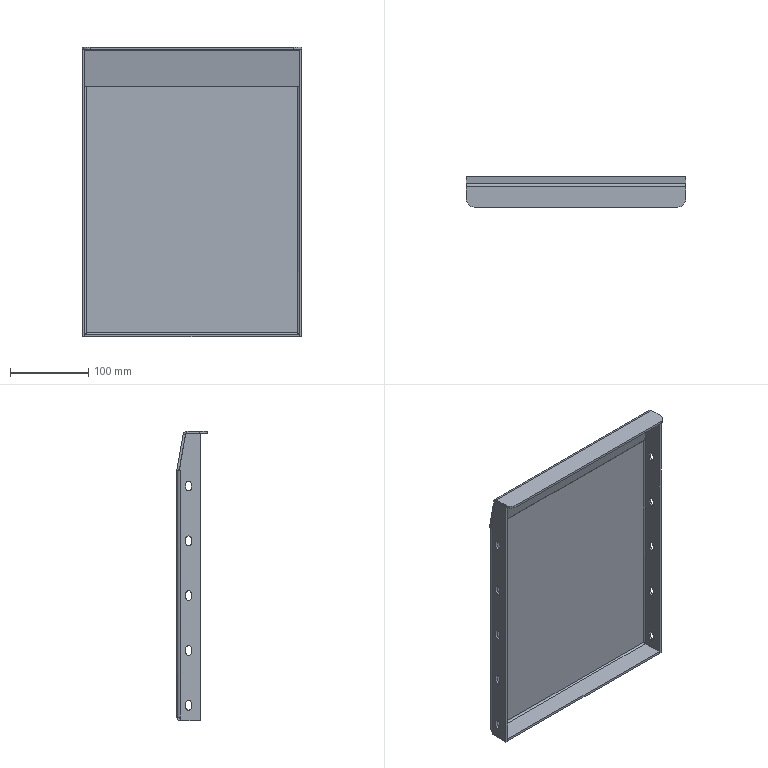Part | SolidWorks | features BaseBody 1 | 1 solid | 116 faces | box 280 x 38.772 x 370.012 mm | volume 407154 mm3 | plane 68 | cylinder 44 | spline 4 | commonest cylinder face diameters 7 x30 4 x7 10 x5 20 x2